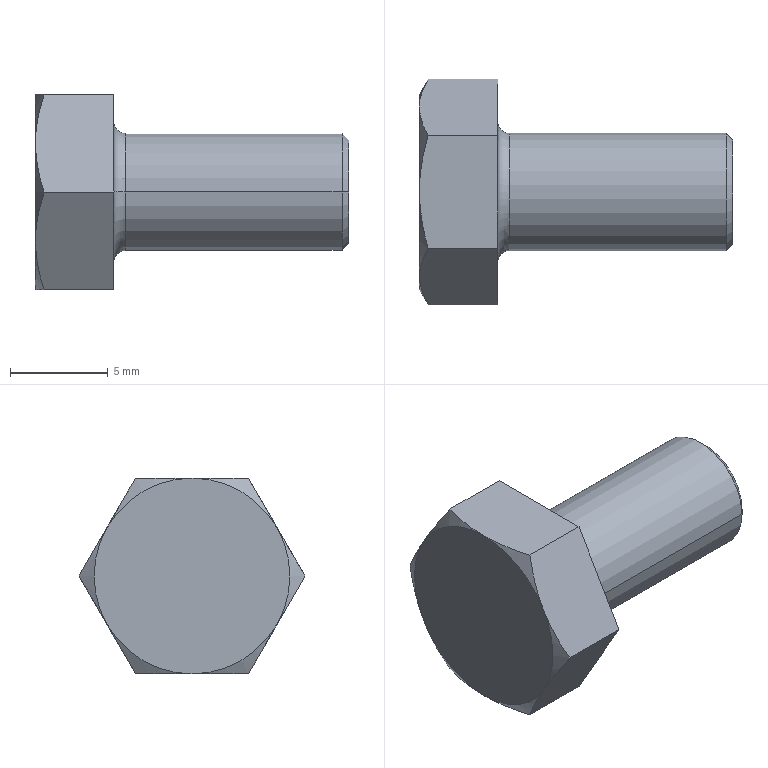Part | SolidWorks | features Chamfer 2, RevCut 2, Revolution 2, Extrusion 1, ICE 1 | 1 solid | 21 faces | box 16 x 11.547 x 10 mm | volume 685.126 mm3 | plane 9 | cone 8 | cylinder 2 | torus 2 | commonest cylinder face diameters 6 x2
STEP:
#1=CARTESIAN_POINT('',(16.,2.667,0.));
#2=VERTEX_POINT('',#1);
#3=CARTESIAN_POINT('',(16.,-2.667,0.));
#4=VERTEX_POINT('',#3);
#5=CARTESIAN_POINT('',(16.,0.,0.));
#6=DIRECTION('',(1.,0.,0.));
#7=DIRECTION('',(0.,-1.,0.));
#8=AXIS2_PLACEMENT_3D('',#5,#6,#7);
#9=CIRCLE('',#8,2.667);
#10=EDGE_CURVE('',#2,#4,#9,.T.);
#11=ORIENTED_EDGE('',*,*,#10,.F.);
#12=CARTESIAN_POINT('',(15.667,3.,0.));
#13=VERTEX_POINT('',#12);
#14=CARTESIAN_POINT('',(15.667,3.,0.));
#15=DIRECTION('',(-0.7071,0.7071,0.));
#16=VECTOR('',#15,1000.);
#17=LINE('',#14,#16);
#18=EDGE_CURVE('',#2,#13,#17,.T.);
#19=ORIENTED_EDGE('',*,*,#18,.T.);
#20=CARTESIAN_POINT('',(15.667,-3.,0.));
#21=VERTEX_POINT('',#20);
#22=CARTESIAN_POINT('',(15.667,0.,0.));
#23=DIRECTION('',(-1.,0.,0.));
#24=DIRECTION('',(0.,-1.,0.));
#25=AXIS2_PLACEMENT_3D('',#22,#23,#24);
#26=CIRCLE('',#25,3.);
#27=EDGE_CURVE('',#21,#13,#26,.T.);
#28=ORIENTED_EDGE('',*,*,#27,.F.);
#29=CARTESIAN_POINT('',(15.667,-3.,0.));
#30=DIRECTION('',(-0.7071,-0.7071,0.));
#31=VECTOR('',#30,1000.);
#32=LINE('',#29,#31);
#33=EDGE_CURVE('',#4,#21,#32,.T.);
#34=ORIENTED_EDGE('',*,*,#33,.F.);
#35=EDGE_LOOP('',(#11,#19,#28,#34));
#36=FACE_OUTER_BOUND('',#35,.T.);
#37=CARTESIAN_POINT('',(15.667,0.,0.));
#38=DIRECTION('',(-1.,0.,0.));
#39=DIRECTION('',(0.,-1.,0.));
#40=AXIS2_PLACEMENT_3D('',#37,#38,#39);
#41=CONICAL_SURFACE('',#40,3.,0.7854);
#42=ADVANCED_FACE('',(#36),#41,.T.);
#43=ORIENTED_EDGE('',*,*,#27,.T.);
#44=CARTESIAN_POINT('',(4.6,3.,0.));
#45=VERTEX_POINT('',#44);
#46=CARTESIAN_POINT('',(4.,3.,0.));
#47=DIRECTION('',(-1.,0.,0.));
#48=VECTOR('',#47,1000.);
#49=LINE('',#46,#48);
#50=EDGE_CURVE('',#13,#45,#49,.T.);
#51=ORIENTED_EDGE('',*,*,#50,.T.);
#52=CARTESIAN_POINT('',(4.6,-3.,0.));
#53=VERTEX_POINT('',#52);
#54=CARTESIAN_POINT('',(4.6,0.,0.));
#55=DIRECTION('',(-1.,0.,0.));
#56=DIRECTION('',(0.,-1.,0.));
#57=AXIS2_PLACEMENT_3D('',#54,#55,#56);
#58=CIRCLE('',#57,3.);
#59=EDGE_CURVE('',#53,#45,#58,.T.);
#60=ORIENTED_EDGE('',*,*,#59,.F.);
#61=CARTESIAN_POINT('',(4.,-3.,0.));
#62=DIRECTION('',(-1.,0.,0.));
#63=VECTOR('',#62,1000.);
#64=LINE('',#61,#63);
#65=EDGE_CURVE('',#21,#53,#64,.T.);
#66=ORIENTED_EDGE('',*,*,#65,.F.);
#67=EDGE_LOOP('',(#43,#51,#60,#66));
#68=FACE_OUTER_BOUND('',#67,.T.);
#69=CARTESIAN_POINT('',(4.,0.,0.));
#70=DIRECTION('',(-1.,0.,0.));
#71=DIRECTION('',(0.,-1.,0.));
#72=AXIS2_PLACEMENT_3D('',#69,#70,#71);
#73=CYLINDRICAL_SURFACE('',#72,3.);
#74=ADVANCED_FACE('',(#68),#73,.T.);
#75=CARTESIAN_POINT('',(4.,3.6,0.));
#76=VERTEX_POINT('',#75);
#77=CARTESIAN_POINT('',(4.,-3.6,0.));
#78=VERTEX_POINT('',#77);
#79=CARTESIAN_POINT('',(4.,0.,0.));
#80=DIRECTION('',(-1.,0.,0.));
#81=DIRECTION('',(0.,-1.,0.));
#82=AXIS2_PLACEMENT_3D('',#79,#80,#81);
#83=CIRCLE('',#82,3.6);
#84=EDGE_CURVE('',#76,#78,#83,.T.);
#85=ORIENTED_EDGE('',*,*,#84,.F.);
#86=CARTESIAN_POINT('',(4.6,3.6,0.));
#87=DIRECTION('',(0.,0.,1.));
#88=DIRECTION('',(0.,-1.,0.));
#89=AXIS2_PLACEMENT_3D('',#86,#87,#88);
#90=CIRCLE('',#89,0.6);
#91=EDGE_CURVE('',#76,#45,#90,.T.);
#92=ORIENTED_EDGE('',*,*,#91,.T.);
#93=CARTESIAN_POINT('',(4.6,0.,0.));
#94=DIRECTION('',(-1.,0.,0.));
#95=DIRECTION('',(0.,-1.,0.));
#96=AXIS2_PLACEMENT_3D('',#93,#94,#95);
#97=CIRCLE('',#96,3.);
#98=EDGE_CURVE('',#45,#53,#97,.T.);
#99=ORIENTED_EDGE('',*,*,#98,.T.);
#100=CARTESIAN_POINT('',(4.6,-3.6,0.));
#101=DIRECTION('',(0.,0.,-1.));
#102=DIRECTION('',(-1.,0.,0.));
#103=AXIS2_PLACEMENT_3D('',#100,#101,#102);
#104=CIRCLE('',#103,0.6);
#105=EDGE_CURVE('',#78,#53,#104,.T.);
#106=ORIENTED_EDGE('',*,*,#105,.F.);
#107=EDGE_LOOP('',(#85,#92,#99,#106));
#108=FACE_OUTER_BOUND('',#107,.T.);
#109=CARTESIAN_POINT('',(4.6,0.,0.));
#110=DIRECTION('',(-1.,0.,0.));
#111=DIRECTION('',(0.,-1.,0.));
#112=AXIS2_PLACEMENT_3D('',#109,#110,#111);
#113=TOROIDAL_SURFACE('',#112,3.6,0.6);
#114=ADVANCED_FACE('',(#108),#113,.F.);
#115=CARTESIAN_POINT('',(4.,-2.887,-5.));
#116=VERTEX_POINT('',#115);
#117=CARTESIAN_POINT('',(4.,2.887,-5.));
#118=VERTEX_POINT('',#117);
#119=CARTESIAN_POINT('',(4.,-2.887,-5.));
#120=DIRECTION('',(0.,1.,0.));
#121=VECTOR('',#120,1000.);
#122=LINE('',#119,#121);
#123=EDGE_CURVE('',#116,#118,#122,.T.);
#124=ORIENTED_EDGE('',*,*,#123,.T.);
#125=CARTESIAN_POINT('',(4.,5.774,0.));
#126=VERTEX_POINT('',#125);
#127=CARTESIAN_POINT('',(4.,2.887,-5.));
#128=DIRECTION('',(0.,0.5,0.866));
#129=VECTOR('',#128,1000.);
#130=LINE('',#127,#129);
#131=EDGE_CURVE('',#118,#126,#130,.T.);
#132=ORIENTED_EDGE('',*,*,#131,.T.);
#133=CARTESIAN_POINT('',(4.,2.887,5.));
#134=VERTEX_POINT('',#133);
#135=CARTESIAN_POINT('',(4.,5.774,0.));
#136=DIRECTION('',(0.,-0.5,0.866));
#137=VECTOR('',#136,1000.);
#138=LINE('',#135,#137);
#139=EDGE_CURVE('',#126,#134,#138,.T.);
#140=ORIENTED_EDGE('',*,*,#139,.T.);
#141=CARTESIAN_POINT('',(4.,-2.887,5.));
#142=VERTEX_POINT('',#141);
#143=CARTESIAN_POINT('',(4.,2.887,5.));
#144=DIRECTION('',(0.,-1.,0.));
#145=VECTOR('',#144,1000.);
#146=LINE('',#143,#145);
#147=EDGE_CURVE('',#134,#142,#146,.T.);
#148=ORIENTED_EDGE('',*,*,#147,.T.);
#149=CARTESIAN_POINT('',(4.,-5.774,0.));
#150=VERTEX_POINT('',#149);
#151=CARTESIAN_POINT('',(4.,-2.887,5.));
#152=DIRECTION('',(0.,-0.5,-0.866));
#153=VECTOR('',#152,1000.);
#154=LINE('',#151,#153);
#155=EDGE_CURVE('',#142,#150,#154,.T.);
#156=ORIENTED_EDGE('',*,*,#155,.T.);
#157=CARTESIAN_POINT('',(4.,-5.774,0.));
#158=DIRECTION('',(0.,0.5,-0.866));
#159=VECTOR('',#158,1000.);
#160=LINE('',#157,#159);
#161=EDGE_CURVE('',#150,#116,#160,.T.);
#162=ORIENTED_EDGE('',*,*,#161,.T.);
#163=EDGE_LOOP('',(#124,#132,#140,#148,#156,#162));
#164=FACE_OUTER_BOUND('',#163,.T.);
#165=CARTESIAN_POINT('',(4.,0.,0.));
#166=DIRECTION('',(-1.,0.,0.));
#167=DIRECTION('',(0.,-1.,0.));
#168=AXIS2_PLACEMENT_3D('',#165,#166,#167);
#169=CIRCLE('',#168,3.6);
#170=EDGE_CURVE('',#78,#76,#169,.T.);
#171=ORIENTED_EDGE('',*,*,#170,.T.);
#172=ORIENTED_EDGE('',*,*,#84,.T.);
#173=EDGE_LOOP('',(#171,#172));
#174=FACE_BOUND('',#173,.T.);
#175=CARTESIAN_POINT('',(4.,2.887,-5.));
#176=DIRECTION('',(1.,0.,0.));
#177=DIRECTION('',(0.,0.,-1.));
#178=AXIS2_PLACEMENT_3D('',#175,#176,#177);
#179=PLANE('',#178);
#180=ADVANCED_FACE('',(#164,#174),#179,.T.);
#181=CARTESIAN_POINT('',(0.4466,2.887,-5.));
#182=VERTEX_POINT('',#181);
#183=CARTESIAN_POINT('',(0.,0.,-5.));
#184=VERTEX_POINT('',#183);
#185=CARTESIAN_POINT('',(0.4466,2.887,-5.));
#186=CARTESIAN_POINT('',(0.3118,2.42,-5.));
#187=CARTESIAN_POINT('',(0.1996,1.947,-5.));
#188=CARTESIAN_POINT('',(0.0431,0.9829,-5.));
#189=CARTESIAN_POINT('',(0.,0.4881,-5.));
#190=CARTESIAN_POINT('',(0.,0.,-5.));
#191=B_SPLINE_CURVE_WITH_KNOTS('',3,(#185,#186,#187,#188,#189,#190),.UNSPECIFIED.,.F.,.F.,(4,2,4),(0.002107,0.003565,0.005022),.UNSPECIFIED.);
#192=EDGE_CURVE('',#182,#184,#191,.T.);
#193=ORIENTED_EDGE('',*,*,#192,.F.);
#194=CARTESIAN_POINT('',(4.,2.887,-5.));
#195=DIRECTION('',(-1.,0.,0.));
#196=VECTOR('',#195,1000.);
#197=LINE('',#194,#196);
#198=EDGE_CURVE('',#118,#182,#197,.T.);
#199=ORIENTED_EDGE('',*,*,#198,.F.);
#200=ORIENTED_EDGE('',*,*,#123,.F.);
#201=CARTESIAN_POINT('',(0.4466,-2.887,-5.));
#202=VERTEX_POINT('',#201);
#203=CARTESIAN_POINT('',(4.,-2.887,-5.));
#204=DIRECTION('',(-1.,0.,0.));
#205=VECTOR('',#204,1000.);
#206=LINE('',#203,#205);
#207=EDGE_CURVE('',#116,#202,#206,.T.);
#208=ORIENTED_EDGE('',*,*,#207,.T.);
#209=CARTESIAN_POINT('',(0.,0.,-5.));
#210=CARTESIAN_POINT('',(0.,-0.4878,-5.));
#211=CARTESIAN_POINT('',(0.04193,-0.9725,-5.));
#212=CARTESIAN_POINT('',(0.1974,-1.936,-5.));
#213=CARTESIAN_POINT('',(0.311,-2.417,-5.));
#214=CARTESIAN_POINT('',(0.4466,-2.887,-5.));
#215=B_SPLINE_CURVE_WITH_KNOTS('',3,(#209,#210,#211,#212,#213,#214),.UNSPECIFIED.,.F.,.F.,(4,2,4),(0.005022,0.006478,0.007935),.UNSPECIFIED.);
#216=EDGE_CURVE('',#184,#202,#215,.T.);
#217=ORIENTED_EDGE('',*,*,#216,.F.);
#218=EDGE_LOOP('',(#193,#199,#200,#208,#217));
#219=FACE_OUTER_BOUND('',#218,.T.);
#220=CARTESIAN_POINT('',(4.,-2.887,-5.));
#221=DIRECTION('',(0.,0.,1.));
#222=DIRECTION('',(0.,-1.,0.));
#223=AXIS2_PLACEMENT_3D('',#220,#221,#222);
#224=PLANE('',#223);
#225=ADVANCED_FACE('',(#219),#224,.F.);
#226=CARTESIAN_POINT('',(0.4466,5.774,0.));
#227=VERTEX_POINT('',#226);
#228=CARTESIAN_POINT('',(0.,4.33,-2.5));
#229=VERTEX_POINT('',#228);
#230=CARTESIAN_POINT('',(0.4466,5.774,0.));
#231=CARTESIAN_POINT('',(0.1739,5.301,-0.8179));
#232=CARTESIAN_POINT('',(0.,4.822,-1.648));
#233=CARTESIAN_POINT('',(0.,4.33,-2.5));
#234=B_SPLINE_CURVE_WITH_KNOTS('',3,(#230,#231,#232,#233),.UNSPECIFIED.,.F.,.F.,(4,4),(0.000000238,0.002921),.UNSPECIFIED.);
#235=EDGE_CURVE('',#227,#229,#234,.T.);
#236=ORIENTED_EDGE('',*,*,#235,.F.);
#237=CARTESIAN_POINT('',(4.,5.774,0.));
#238=DIRECTION('',(-1.,0.,0.));
#239=VECTOR('',#238,1000.);
#240=LINE('',#237,#239);
#241=EDGE_CURVE('',#126,#227,#240,.T.);
#242=ORIENTED_EDGE('',*,*,#241,.F.);
#243=ORIENTED_EDGE('',*,*,#131,.F.);
#244=ORIENTED_EDGE('',*,*,#198,.T.);
#245=CARTESIAN_POINT('',(0.,4.33,-2.5));
#246=CARTESIAN_POINT('',(0.,4.208,-2.712));
#247=CARTESIAN_POINT('',(0.01056,4.085,-2.925));
#248=CARTESIAN_POINT('',(0.0514,3.841,-3.347));
#249=CARTESIAN_POINT('',(0.08166,3.72,-3.556));
#250=CARTESIAN_POINT('',(0.1983,3.36,-4.181));
#251=CARTESIAN_POINT('',(0.3106,3.122,-4.592));
#252=CARTESIAN_POINT('',(0.4466,2.887,-5.));
#253=B_SPLINE_CURVE_WITH_KNOTS('',3,(#245,#246,#247,#248,#249,#250,#251,#252),.UNSPECIFIED.,.F.,.F.,(4,2,2,4),(0.002921,0.003649,0.004376,0.005831),.UNSPECIFIED.);
#254=EDGE_CURVE('',#229,#182,#253,.T.);
#255=ORIENTED_EDGE('',*,*,#254,.F.);
#256=EDGE_LOOP('',(#236,#242,#243,#244,#255));
#257=FACE_OUTER_BOUND('',#256,.T.);
#258=CARTESIAN_POINT('',(4.,2.887,-5.));
#259=DIRECTION('',(0.,-0.866,0.5));
#260=DIRECTION('',(0.,-0.5,-0.866));
#261=AXIS2_PLACEMENT_3D('',#258,#259,#260);
#262=PLANE('',#261);
#263=ADVANCED_FACE('',(#257),#262,.F.);
#264=CARTESIAN_POINT('',(0.4466,2.887,5.));
#265=VERTEX_POINT('',#264);
#266=CARTESIAN_POINT('',(0.,4.33,2.5));
#267=VERTEX_POINT('',#266);
#268=CARTESIAN_POINT('',(0.4466,2.887,5.));
#269=CARTESIAN_POINT('',(0.1739,3.359,4.182));
#270=CARTESIAN_POINT('',(0.,3.838,3.352));
#271=CARTESIAN_POINT('',(0.,4.33,2.5));
#272=B_SPLINE_CURVE_WITH_KNOTS('',3,(#268,#269,#270,#271),.UNSPECIFIED.,.F.,.F.,(4,4),(0.000000238,0.002921),.UNSPECIFIED.);
#273=EDGE_CURVE('',#265,#267,#272,.T.);
#274=ORIENTED_EDGE('',*,*,#273,.F.);
#275=CARTESIAN_POINT('',(4.,2.887,5.));
#276=DIRECTION('',(-1.,0.,0.));
#277=VECTOR('',#276,1000.);
#278=LINE('',#275,#277);
#279=EDGE_CURVE('',#134,#265,#278,.T.);
#280=ORIENTED_EDGE('',*,*,#279,.F.);
#281=ORIENTED_EDGE('',*,*,#139,.F.);
#282=ORIENTED_EDGE('',*,*,#241,.T.);
#283=CARTESIAN_POINT('',(0.,4.33,2.5));
#284=CARTESIAN_POINT('',(0.,4.453,2.288));
#285=CARTESIAN_POINT('',(0.01056,4.576,2.075));
#286=CARTESIAN_POINT('',(0.0514,4.819,1.653));
#287=CARTESIAN_POINT('',(0.08166,4.94,1.444));
#288=CARTESIAN_POINT('',(0.1983,5.3,0.8193));
#289=CARTESIAN_POINT('',(0.3106,5.538,0.4079));
#290=CARTESIAN_POINT('',(0.4466,5.774,0.));
#291=B_SPLINE_CURVE_WITH_KNOTS('',3,(#283,#284,#285,#286,#287,#288,#289,#290),.UNSPECIFIED.,.F.,.F.,(4,2,2,4),(0.002921,0.003649,0.004376,0.005831),.UNSPECIFIED.);
#292=EDGE_CURVE('',#267,#227,#291,.T.);
#293=ORIENTED_EDGE('',*,*,#292,.F.);
#294=EDGE_LOOP('',(#274,#280,#281,#282,#293));
#295=FACE_OUTER_BOUND('',#294,.T.);
#296=CARTESIAN_POINT('',(4.,5.774,0.));
#297=DIRECTION('',(0.,-0.866,-0.5));
#298=DIRECTION('',(0.,0.5,-0.866));
#299=AXIS2_PLACEMENT_3D('',#296,#297,#298);
#300=PLANE('',#299);
#301=ADVANCED_FACE('',(#295),#300,.F.);
#302=CARTESIAN_POINT('',(0.4466,-2.887,5.));
#303=VERTEX_POINT('',#302);
#304=CARTESIAN_POINT('',(0.,0.,5.));
#305=VERTEX_POINT('',#304);
#306=CARTESIAN_POINT('',(0.4466,-2.887,5.));
#307=CARTESIAN_POINT('',(0.311,-2.417,5.));
#308=CARTESIAN_POINT('',(0.1974,-1.936,5.));
#309=CARTESIAN_POINT('',(0.04193,-0.9725,5.));
#310=CARTESIAN_POINT('',(0.,-0.4878,5.));
#311=CARTESIAN_POINT('',(0.,0.,5.));
#312=B_SPLINE_CURVE_WITH_KNOTS('',3,(#306,#307,#308,#309,#310,#311),.UNSPECIFIED.,.F.,.F.,(4,2,4),(0.005159,0.006619,0.008079),.UNSPECIFIED.);
#313=EDGE_CURVE('',#303,#305,#312,.T.);
#314=ORIENTED_EDGE('',*,*,#313,.F.);
#315=CARTESIAN_POINT('',(4.,-2.887,5.));
#316=DIRECTION('',(-1.,0.,0.));
#317=VECTOR('',#316,1000.);
#318=LINE('',#315,#317);
#319=EDGE_CURVE('',#142,#303,#318,.T.);
#320=ORIENTED_EDGE('',*,*,#319,.F.);
#321=ORIENTED_EDGE('',*,*,#147,.F.);
#322=ORIENTED_EDGE('',*,*,#279,.T.);
#323=CARTESIAN_POINT('',(0.,0.,5.));
#324=CARTESIAN_POINT('',(0.,0.4881,5.));
#325=CARTESIAN_POINT('',(0.0431,0.9829,5.));
#326=CARTESIAN_POINT('',(0.1996,1.947,5.));
#327=CARTESIAN_POINT('',(0.3118,2.42,5.));
#328=CARTESIAN_POINT('',(0.4466,2.887,5.));
#329=B_SPLINE_CURVE_WITH_KNOTS('',3,(#323,#324,#325,#326,#327,#328),.UNSPECIFIED.,.F.,.F.,(4,2,4),(0.008079,0.00954,0.011),.UNSPECIFIED.);
#330=EDGE_CURVE('',#305,#265,#329,.T.);
#331=ORIENTED_EDGE('',*,*,#330,.F.);
#332=EDGE_LOOP('',(#314,#320,#321,#322,#331));
#333=FACE_OUTER_BOUND('',#332,.T.);
#334=CARTESIAN_POINT('',(4.,2.887,5.));
#335=DIRECTION('',(0.,0.,-1.));
#336=DIRECTION('',(-1.,0.,0.));
#337=AXIS2_PLACEMENT_3D('',#334,#335,#336);
#338=PLANE('',#337);
#339=ADVANCED_FACE('',(#333),#338,.F.);
#340=CARTESIAN_POINT('',(0.4466,-5.774,0.));
#341=VERTEX_POINT('',#340);
#342=CARTESIAN_POINT('',(0.,-4.33,2.5));
#343=VERTEX_POINT('',#342);
#344=CARTESIAN_POINT('',(0.4466,-5.774,0.));
#345=CARTESIAN_POINT('',(0.1739,-5.301,0.8179));
#346=CARTESIAN_POINT('',(0.,-4.822,1.648));
#347=CARTESIAN_POINT('',(0.,-4.33,2.5));
#348=B_SPLINE_CURVE_WITH_KNOTS('',3,(#344,#345,#346,#347),.UNSPECIFIED.,.F.,.F.,(4,4),(0.000000238,0.002921),.UNSPECIFIED.);
#349=EDGE_CURVE('',#341,#343,#348,.T.);
#350=ORIENTED_EDGE('',*,*,#349,.F.);
#351=CARTESIAN_POINT('',(4.,-5.774,0.));
#352=DIRECTION('',(-1.,0.,0.));
#353=VECTOR('',#352,1000.);
#354=LINE('',#351,#353);
#355=EDGE_CURVE('',#150,#341,#354,.T.);
#356=ORIENTED_EDGE('',*,*,#355,.F.);
#357=ORIENTED_EDGE('',*,*,#155,.F.);
#358=ORIENTED_EDGE('',*,*,#319,.T.);
#359=CARTESIAN_POINT('',(0.,-4.33,2.5));
#360=CARTESIAN_POINT('',(0.,-4.208,2.712));
#361=CARTESIAN_POINT('',(0.01056,-4.085,2.925));
#362=CARTESIAN_POINT('',(0.0514,-3.841,3.347));
#363=CARTESIAN_POINT('',(0.08166,-3.72,3.556));
#364=CARTESIAN_POINT('',(0.1983,-3.36,4.181));
#365=CARTESIAN_POINT('',(0.3106,-3.122,4.592));
#366=CARTESIAN_POINT('',(0.4466,-2.887,5.));
#367=B_SPLINE_CURVE_WITH_KNOTS('',3,(#359,#360,#361,#362,#363,#364,#365,#366),.UNSPECIFIED.,.F.,.F.,(4,2,2,4),(0.002921,0.003649,0.004376,0.005831),.UNSPECIFIED.);
#368=EDGE_CURVE('',#343,#303,#367,.T.);
#369=ORIENTED_EDGE('',*,*,#368,.F.);
#370=EDGE_LOOP('',(#350,#356,#357,#358,#369));
#371=FACE_OUTER_BOUND('',#370,.T.);
#372=CARTESIAN_POINT('',(4.,-2.887,5.));
#373=DIRECTION('',(0.,0.866,-0.5));
#374=DIRECTION('',(0.,0.5,0.866));
#375=AXIS2_PLACEMENT_3D('',#372,#373,#374);
#376=PLANE('',#375);
#377=ADVANCED_FACE('',(#371),#376,.F.);
#378=CARTESIAN_POINT('',(0.,-4.33,-2.5));
#379=VERTEX_POINT('',#378);
#380=CARTESIAN_POINT('',(0.4466,-2.887,-5.));
#381=CARTESIAN_POINT('',(0.1739,-3.359,-4.182));
#382=CARTESIAN_POINT('',(0.,-3.838,-3.352));
#383=CARTESIAN_POINT('',(0.,-4.33,-2.5));
#384=B_SPLINE_CURVE_WITH_KNOTS('',3,(#380,#381,#382,#383),.UNSPECIFIED.,.F.,.F.,(4,4),(0.000000238,0.002921),.UNSPECIFIED.);
#385=EDGE_CURVE('',#202,#379,#384,.T.);
#386=ORIENTED_EDGE('',*,*,#385,.F.);
#387=ORIENTED_EDGE('',*,*,#207,.F.);
#388=ORIENTED_EDGE('',*,*,#161,.F.);
#389=ORIENTED_EDGE('',*,*,#355,.T.);
#390=CARTESIAN_POINT('',(0.,-4.33,-2.5));
#391=CARTESIAN_POINT('',(0.,-4.453,-2.288));
#392=CARTESIAN_POINT('',(0.01056,-4.576,-2.075));
#393=CARTESIAN_POINT('',(0.0514,-4.819,-1.653));
#394=CARTESIAN_POINT('',(0.08166,-4.94,-1.444));
#395=CARTESIAN_POINT('',(0.1983,-5.3,-0.8193));
#396=CARTESIAN_POINT('',(0.3106,-5.538,-0.4079));
#397=CARTESIAN_POINT('',(0.4466,-5.774,0.));
#398=B_SPLINE_CURVE_WITH_KNOTS('',3,(#390,#391,#392,#393,#394,#395,#396,#397),.UNSPECIFIED.,.F.,.F.,(4,2,2,4),(0.002921,0.003649,0.004376,0.005831),.UNSPECIFIED.);
#399=EDGE_CURVE('',#379,#341,#398,.T.);
#400=ORIENTED_EDGE('',*,*,#399,.F.);
#401=EDGE_LOOP('',(#386,#387,#388,#389,#400));
#402=FACE_OUTER_BOUND('',#401,.T.);
#403=CARTESIAN_POINT('',(4.,-5.774,0.));
#404=DIRECTION('',(0.,0.866,0.5));
#405=DIRECTION('',(0.,-0.5,0.866));
#406=AXIS2_PLACEMENT_3D('',#403,#404,#405);
#407=PLANE('',#406);
#408=ADVANCED_FACE('',(#402),#407,.F.);
#409=ORIENTED_EDGE('',*,*,#216,.T.);
#410=ORIENTED_EDGE('',*,*,#385,.T.);
#411=CARTESIAN_POINT('',(0.,0.,0.));
#412=DIRECTION('',(1.,0.,0.));
#413=DIRECTION('',(0.,0.,-1.));
#414=AXIS2_PLACEMENT_3D('',#411,#412,#413);
#415=CIRCLE('',#414,5.);
#416=EDGE_CURVE('',#379,#184,#415,.T.);
#417=ORIENTED_EDGE('',*,*,#416,.T.);
#418=EDGE_LOOP('',(#409,#410,#417));
#419=FACE_OUTER_BOUND('',#418,.T.);
#420=CARTESIAN_POINT('',(0.,0.,0.));
#421=DIRECTION('',(1.,0.,0.));
#422=DIRECTION('',(0.,0.,1.));
#423=AXIS2_PLACEMENT_3D('',#420,#421,#422);
#424=CONICAL_SURFACE('',#423,5.,1.047);
#425=ADVANCED_FACE('',(#419),#424,.T.);
#426=ORIENTED_EDGE('',*,*,#349,.T.);
#427=CARTESIAN_POINT('',(0.,0.,0.));
#428=DIRECTION('',(1.,0.,0.));
#429=DIRECTION('',(0.,0.,-1.));
#430=AXIS2_PLACEMENT_3D('',#427,#428,#429);
#431=CIRCLE('',#430,5.);
#432=EDGE_CURVE('',#343,#379,#431,.T.);
#433=ORIENTED_EDGE('',*,*,#432,.T.);
#434=ORIENTED_EDGE('',*,*,#399,.T.);
#435=EDGE_LOOP('',(#426,#433,#434));
#436=FACE_OUTER_BOUND('',#435,.T.);
#437=CARTESIAN_POINT('',(0.,0.,0.));
#438=DIRECTION('',(1.,0.,0.));
#439=DIRECTION('',(0.,0.,1.));
#440=AXIS2_PLACEMENT_3D('',#437,#438,#439);
#441=CONICAL_SURFACE('',#440,5.,1.047);
#442=ADVANCED_FACE('',(#436),#441,.T.);
#443=ORIENTED_EDGE('',*,*,#313,.T.);
#444=CARTESIAN_POINT('',(0.,0.,0.));
#445=DIRECTION('',(1.,0.,0.));
#446=DIRECTION('',(0.,0.,-1.));
#447=AXIS2_PLACEMENT_3D('',#444,#445,#446);
#448=CIRCLE('',#447,5.);
#449=EDGE_CURVE('',#305,#343,#448,.T.);
#450=ORIENTED_EDGE('',*,*,#449,.T.);
#451=ORIENTED_EDGE('',*,*,#368,.T.);
#452=EDGE_LOOP('',(#443,#450,#451));
#453=FACE_OUTER_BOUND('',#452,.T.);
#454=CARTESIAN_POINT('',(0.,0.,0.));
#455=DIRECTION('',(1.,0.,0.));
#456=DIRECTION('',(0.,0.,1.));
#457=AXIS2_PLACEMENT_3D('',#454,#455,#456);
#458=CONICAL_SURFACE('',#457,5.,1.047);
#459=ADVANCED_FACE('',(#453),#458,.T.);
#460=ORIENTED_EDGE('',*,*,#273,.T.);
#461=CARTESIAN_POINT('',(0.,0.,0.));
#462=DIRECTION('',(-1.,0.,0.));
#463=DIRECTION('',(0.,0.,1.));
#464=AXIS2_PLACEMENT_3D('',#461,#462,#463);
#465=CIRCLE('',#464,5.);
#466=EDGE_CURVE('',#305,#267,#465,.T.);
#467=ORIENTED_EDGE('',*,*,#466,.F.);
#468=ORIENTED_EDGE('',*,*,#330,.T.);
#469=EDGE_LOOP('',(#460,#467,#468));
#470=FACE_OUTER_BOUND('',#469,.T.);
#471=CARTESIAN_POINT('',(0.,0.,0.));
#472=DIRECTION('',(1.,0.,0.));
#473=DIRECTION('',(0.,0.,1.));
#474=AXIS2_PLACEMENT_3D('',#471,#472,#473);
#475=CONICAL_SURFACE('',#474,5.,1.047);
#476=ADVANCED_FACE('',(#470),#475,.T.);
#477=ORIENTED_EDGE('',*,*,#292,.T.);
#478=ORIENTED_EDGE('',*,*,#235,.T.);
#479=CARTESIAN_POINT('',(0.,0.,0.));
#480=DIRECTION('',(1.,0.,0.));
#481=DIRECTION('',(0.,0.,-1.));
#482=AXIS2_PLACEMENT_3D('',#479,#480,#481);
#483=CIRCLE('',#482,5.);
#484=EDGE_CURVE('',#229,#267,#483,.T.);
#485=ORIENTED_EDGE('',*,*,#484,.T.);
#486=EDGE_LOOP('',(#477,#478,#485));
#487=FACE_OUTER_BOUND('',#486,.T.);
#488=CARTESIAN_POINT('',(0.,0.,0.));
#489=DIRECTION('',(1.,0.,0.));
#490=DIRECTION('',(0.,0.,1.));
#491=AXIS2_PLACEMENT_3D('',#488,#489,#490);
#492=CONICAL_SURFACE('',#491,5.,1.047);
#493=ADVANCED_FACE('',(#487),#492,.T.);
#494=ORIENTED_EDGE('',*,*,#254,.T.);
#495=ORIENTED_EDGE('',*,*,#192,.T.);
#496=CARTESIAN_POINT('',(0.,0.,0.));
#497=DIRECTION('',(1.,0.,0.));
#498=DIRECTION('',(0.,0.,-1.));
#499=AXIS2_PLACEMENT_3D('',#496,#497,#498);
#500=CIRCLE('',#499,5.);
#501=EDGE_CURVE('',#184,#229,#500,.T.);
#502=ORIENTED_EDGE('',*,*,#501,.T.);
#503=EDGE_LOOP('',(#494,#495,#502));
#504=FACE_OUTER_BOUND('',#503,.T.);
#505=CARTESIAN_POINT('',(0.,0.,0.));
#506=DIRECTION('',(1.,0.,0.));
#507=DIRECTION('',(0.,0.,1.));
#508=AXIS2_PLACEMENT_3D('',#505,#506,#507);
#509=CONICAL_SURFACE('',#508,5.,1.047);
#510=ADVANCED_FACE('',(#504),#509,.T.);
#511=ORIENTED_EDGE('',*,*,#501,.F.);
#512=ORIENTED_EDGE('',*,*,#416,.F.);
#513=ORIENTED_EDGE('',*,*,#432,.F.);
#514=ORIENTED_EDGE('',*,*,#449,.F.);
#515=ORIENTED_EDGE('',*,*,#466,.T.);
#516=ORIENTED_EDGE('',*,*,#484,.F.);
#517=EDGE_LOOP('',(#511,#512,#513,#514,#515,#516));
#518=FACE_OUTER_BOUND('',#517,.T.);
#519=CARTESIAN_POINT('',(0.,2.887,-5.));
#520=DIRECTION('',(1.,0.,0.));
#521=DIRECTION('',(0.,0.,-1.));
#522=AXIS2_PLACEMENT_3D('',#519,#520,#521);
#523=PLANE('',#522);
#524=ADVANCED_FACE('',(#518),#523,.F.);
#525=ORIENTED_EDGE('',*,*,#91,.F.);
#526=ORIENTED_EDGE('',*,*,#170,.F.);
#527=ORIENTED_EDGE('',*,*,#105,.T.);
#528=ORIENTED_EDGE('',*,*,#59,.T.);
#529=EDGE_LOOP('',(#525,#526,#527,#528));
#530=FACE_OUTER_BOUND('',#529,.T.);
#531=CARTESIAN_POINT('',(4.6,0.,0.));
#532=DIRECTION('',(-1.,0.,0.));
#533=DIRECTION('',(0.,-1.,0.));
#534=AXIS2_PLACEMENT_3D('',#531,#532,#533);
#535=TOROIDAL_SURFACE('',#534,3.6,0.6);
#536=ADVANCED_FACE('',(#530),#535,.F.);
#537=CARTESIAN_POINT('',(16.,0.,0.));
#538=DIRECTION('',(1.,0.,0.));
#539=DIRECTION('',(0.,-1.,0.));
#540=AXIS2_PLACEMENT_3D('',#537,#538,#539);
#541=CIRCLE('',#540,2.667);
#542=EDGE_CURVE('',#4,#2,#541,.T.);
#543=ORIENTED_EDGE('',*,*,#542,.T.);
#544=ORIENTED_EDGE('',*,*,#10,.T.);
#545=EDGE_LOOP('',(#543,#544));
#546=FACE_OUTER_BOUND('',#545,.T.);
#547=CARTESIAN_POINT('',(16.,3.,0.));
#548=DIRECTION('',(-1.,0.,0.));
#549=DIRECTION('',(0.,-1.,0.));
#550=AXIS2_PLACEMENT_3D('',#547,#548,#549);
#551=PLANE('',#550);
#552=ADVANCED_FACE('',(#546),#551,.F.);
#553=ORIENTED_EDGE('',*,*,#50,.F.);
#554=CARTESIAN_POINT('',(15.667,0.,0.));
#555=DIRECTION('',(-1.,0.,0.));
#556=DIRECTION('',(0.,-1.,0.));
#557=AXIS2_PLACEMENT_3D('',#554,#555,#556);
#558=CIRCLE('',#557,3.);
#559=EDGE_CURVE('',#13,#21,#558,.T.);
#560=ORIENTED_EDGE('',*,*,#559,.T.);
#561=ORIENTED_EDGE('',*,*,#65,.T.);
#562=ORIENTED_EDGE('',*,*,#98,.F.);
#563=EDGE_LOOP('',(#553,#560,#561,#562));
#564=FACE_OUTER_BOUND('',#563,.T.);
#565=CARTESIAN_POINT('',(4.,0.,0.));
#566=DIRECTION('',(-1.,0.,0.));
#567=DIRECTION('',(0.,-1.,0.));
#568=AXIS2_PLACEMENT_3D('',#565,#566,#567);
#569=CYLINDRICAL_SURFACE('',#568,3.);
#570=ADVANCED_FACE('',(#564),#569,.T.);
#571=ORIENTED_EDGE('',*,*,#18,.F.);
#572=ORIENTED_EDGE('',*,*,#542,.F.);
#573=ORIENTED_EDGE('',*,*,#33,.T.);
#574=ORIENTED_EDGE('',*,*,#559,.F.);
#575=EDGE_LOOP('',(#571,#572,#573,#574));
#576=FACE_OUTER_BOUND('',#575,.T.);
#577=CARTESIAN_POINT('',(15.667,0.,0.));
#578=DIRECTION('',(-1.,0.,0.));
#579=DIRECTION('',(0.,-1.,0.));
#580=AXIS2_PLACEMENT_3D('',#577,#578,#579);
#581=CONICAL_SURFACE('',#580,3.,0.7854);
#582=ADVANCED_FACE('',(#576),#581,.T.);
#583=CLOSED_SHELL('',(#42,#74,#114,#180,#225,#263,#301,#339,#377,#408,#425,#442,#459,#476,#493,#510,#524,#536,#552,#570,#582));
#584=MANIFOLD_SOLID_BREP('',#583);
#585=CARTESIAN_POINT('',(0.,0.,0.));
#586=DIRECTION('',(0.,0.,1.));
#587=DIRECTION('',(1.,0.,0.));
#588=AXIS2_PLACEMENT_3D('',#585,#586,#587);
#589=(LENGTH_UNIT()NAMED_UNIT(*)SI_UNIT(.MILLI.,.METRE.));
#590=UNCERTAINTY_MEASURE_WITH_UNIT(LENGTH_MEASURE(0.00001),#589,'','');
#591=(NAMED_UNIT(*)PLANE_ANGLE_UNIT()SI_UNIT($,.RADIAN.));
#592=(NAMED_UNIT(*)SI_UNIT($,.STERADIAN.)SOLID_ANGLE_UNIT());
#593=(GEOMETRIC_REPRESENTATION_CONTEXT(3)GLOBAL_UNCERTAINTY_ASSIGNED_CONTEXT((#590))GLOBAL_UNIT_ASSIGNED_CONTEXT((#589,#591,#592))REPRESENTATION_CONTEXT('',''));
#594=ADVANCED_BREP_SHAPE_REPRESENTATION('',(#584,#588),#593);